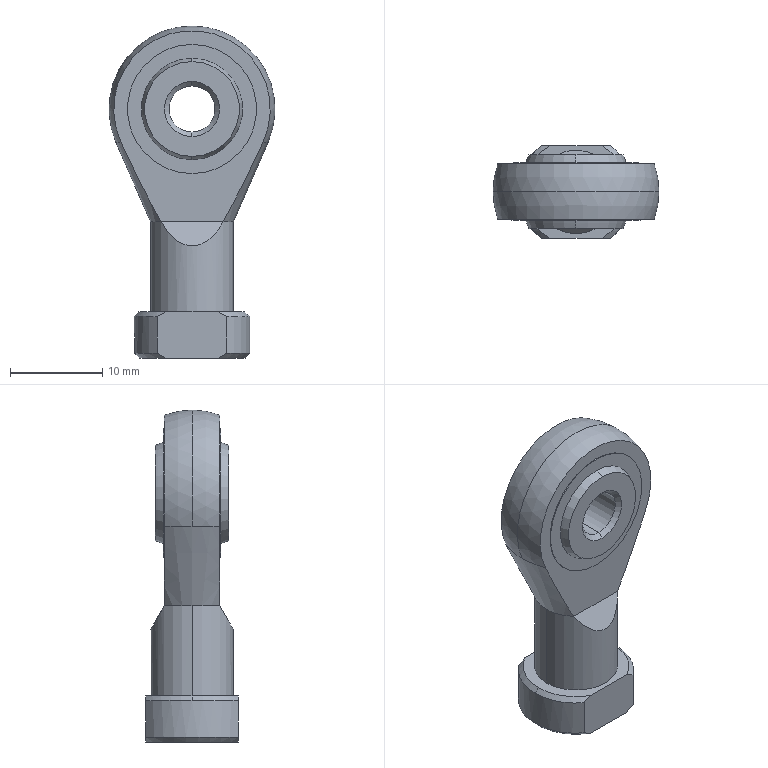Part | STEP file | 001-004-F_M5X080U | 1 solid | 48 faces | box 18 x 10 x 36 mm | volume 2763 mm3 | cone 17 | cylinder 13 | plane 12 | other 4 | sphere 2 | commonest cylinder face diameters 14 x4 12.5 x3 4.134 x2 5 x2 9 x2